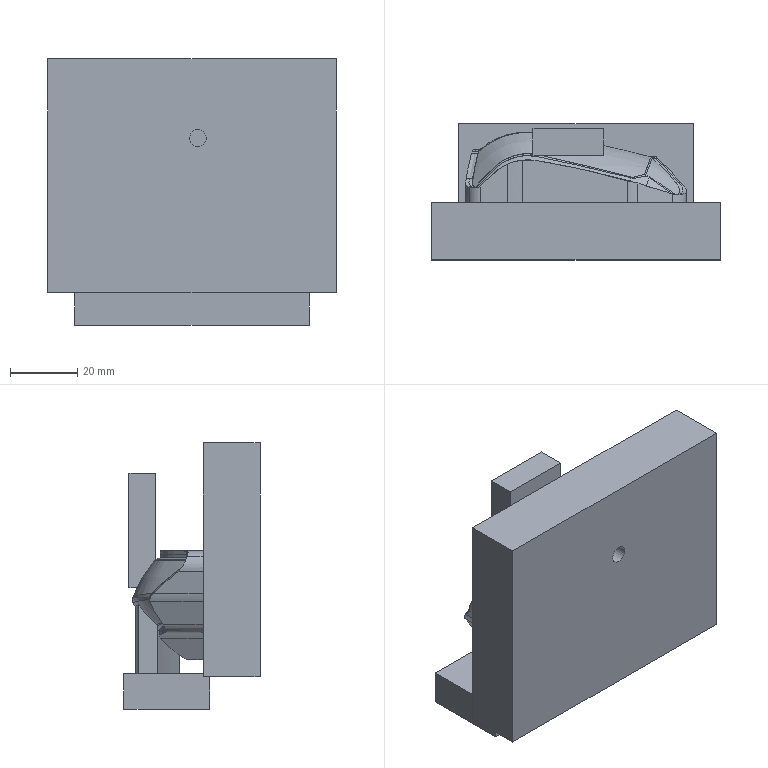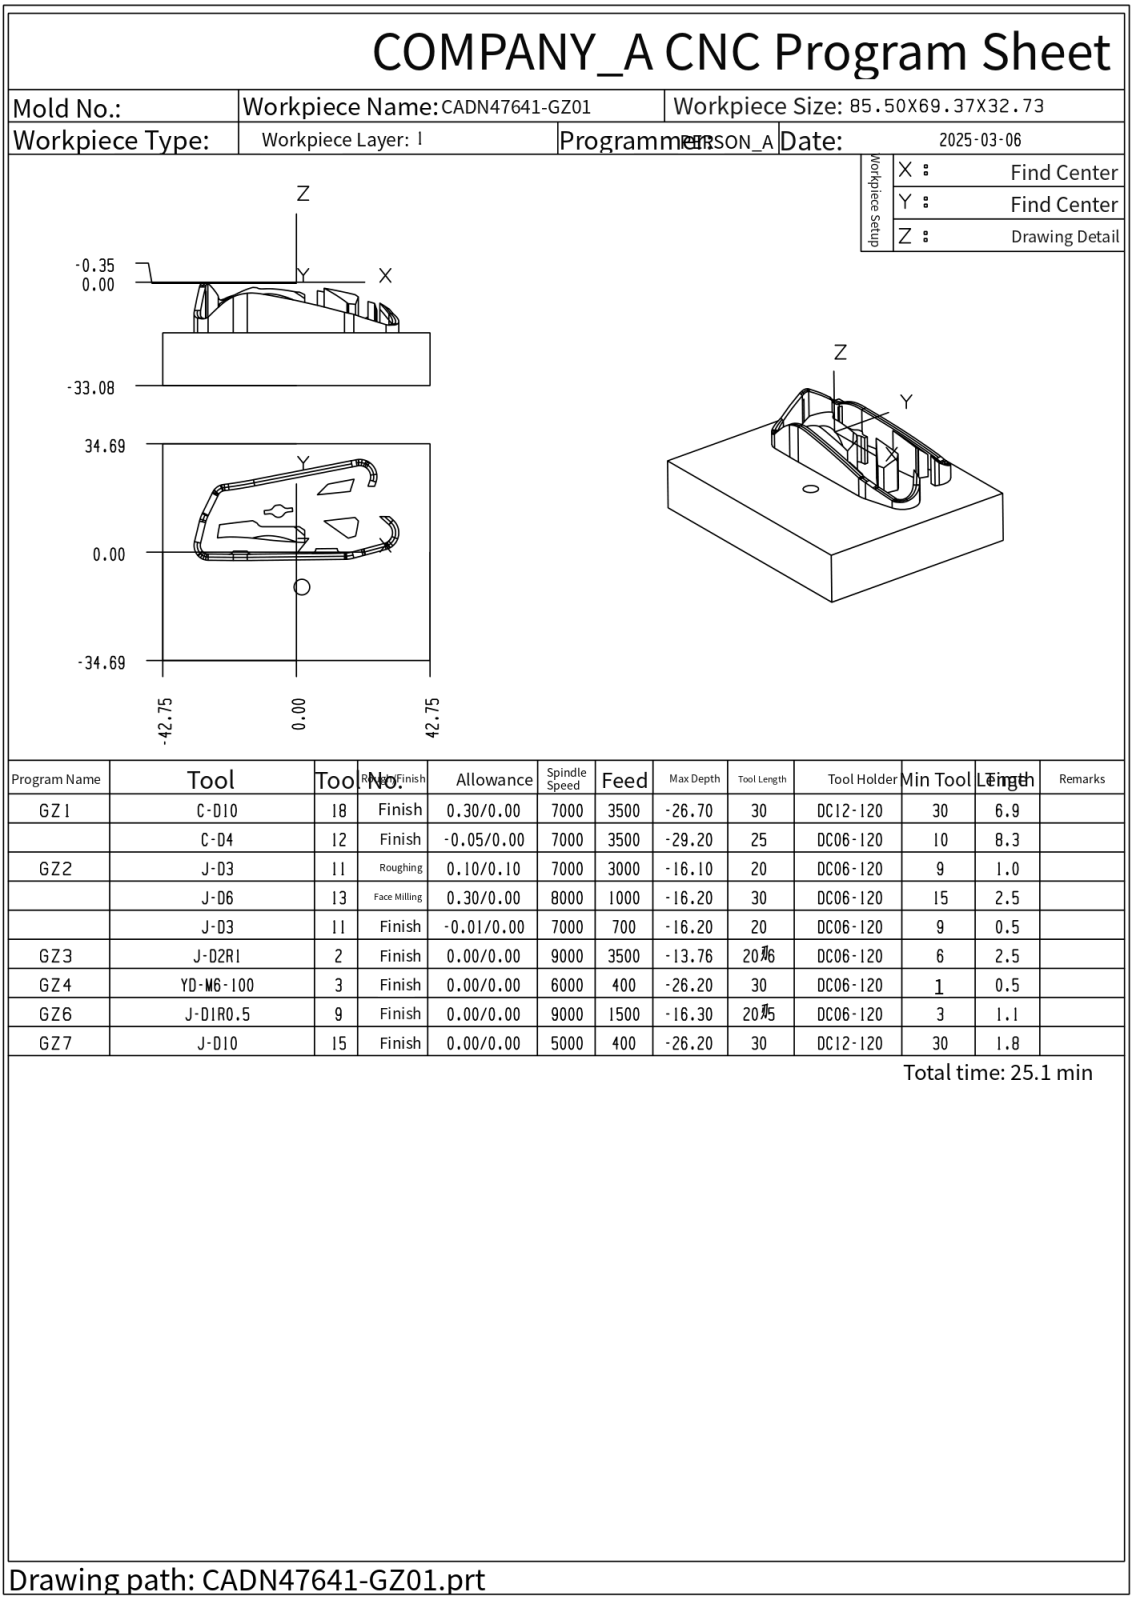NC program | NX | posted by the shop | part box 85.5 x 40.385 x 79 mm
Lines 1 to 894 of 71032:
1 BEGIN PGM A MM
2 BLK FORM 0.1 Z X-200 Y-200 Z-20
3 BLK FORM 0.2  X+200  Y+200  Z+0
4 CYCL DEF 247 DATUM SETTING ~
Q339=+1
5 * - OPERATION: 动态开粗_COPY_1 - TOOL: T14 C-D8
6 M5
7 M9
8 PLANE RESET STAY
9 CALL LBL100
10 ;(C-D8 D=8. R=0.)
11 M01
12 TOOL CALL 14 Z S7000
13 CALL LBL101
14 M3 M8
15 M51
16 CYCL DEF 7.0
17 CYCL DEF 7.1 X0
18 CYCL DEF 7.2 Y0
19 CYCL DEF 7.3 Z0
20 CYCL DEF 32.0 TOLERANCE
21 CYCL DEF 32.1 T0.096
22 CYCL DEF 32.2 HSC-MODE:0
23 L M126
24 L A+0.0 C+0.0 FMAX
25 L X-40.7663 Y-4.7564 FMAX
26 L Z5.3 FMAX
27 L Z-14.7 FMAX
28 L Z-17.7 F4000.
29 L X-40.0254 Y-4.7388
30 L X-39.2862 Y-4.6863
31 CC X-39.5061 Y-3.8936
32 C X-38.7492 Y-4.216 DR+
33 CC X-55.9353 Y-.1596
34 C X-38.2866 Y.4217 DR+
35 L X-38.2031 Y11.2888
36 CC X-33.0151 Y10.2125
37 C X-34.5468 Y15.2848 DR-
38 CC X-28.8054 Y-3.3134
39 C X-28.3228 Y16.1449 DR-
40 L X-19.7606 Y16.191
41 L X33.2624 Y16.1529
42 CC X32.3188 Y11.0031
43 C X37.3148 Y12.5687 DR-
44 CC X19.5711 Y6.8917
45 C X38.1961 Y6.4747 DR-
46 CC X-682.1256 Y-2.6235
47 C X38.2015 Y-11.2855 DR-
48 CC X33.0063 Y-10.2087
49 C X34.5482 Y-15.2853 DR-
50 CC X28.812 Y3.2985
51 C X28.3241 Y-16.1444 DR-
52 L X19.7619 Y-16.1904
53 L X-33.261 Y-16.1559
54 CC X-32.3254 Y-11.0212
55 C X-37.2907 Y-12.6294 DR-
56 CC X-19.0827 Y-6.7608
57 C X-38.1116 Y-4.7925 DR-
58 CC X-207.714 Y6.8756
59 C X-37.7288 Y9.353 DR+
60 CC X-31.4594 Y8.5945
61 C X-33.4511 Y14.5873 DR-
62 CC X-26.9702 Y-4.9504
63 C X-26.565 Y15.6302 DR-
64 L X-17.6279 Y15.6907
65 L X31.6049 Y15.6508
66 CC X30.5961 Y9.326
67 C X36.7188 Y11.2056 DR-
68 CC X15.2296 Y4.6174
69 C X37.699 Y4.0555 DR-
70 CC X-599.7023 Y-3.1683
71 C X37.708 Y-9.5448 DR-
72 CC X31.4132 Y-8.555
73 C X33.3692 Y-14.6195 DR-
74 CC X27.0224 Y4.8766
75 C X26.7268 Y-15.6245 DR-
76 L X17.9148 Y-15.69
77 L X-31.6032 Y-15.6509
78 CC X-30.5967 Y-9.3279
79 C X-36.7142 Y-11.2172 DR-
80 CC X-19.4868 Y-5.7072
81 C X-37.4871 Y-3.9371 DR-
82 CC X-490.3806 Y12.528
83 C X-37.2095 Y8.1065 DR+
84 CC X-30.1497 Y7.2716
85 C X-32.3545 Y14.0301 DR-
86 CC X-25.5192 Y-6.9093
87 C X-25.2814 Y15.1162 DR-
88 L X-15.5946 Y15.1904
89 L X30.0422 Y15.1602
90 CC X29.3483 Y8.1097
91 C X36.0839 Y10.3054 DR-
92 CC X14.3082 Y3.2829
93 C X37.1843 Y2.8563 DR-
94 CC X-145.6723 Y-2.6925
95 C X37.1816 Y-8.3282 DR-
96 CC X30.0937 Y-7.2324
97 C X32.2692 Y-14.0666 DR-
98 CC X25.3235 Y8.0785
99 C X24.9413 Y-15.1271 DR-
100 L X16.6293 Y-15.1895
101 L X-30.0076 Y-15.1621
102 CC X-29.3404 Y-8.0931
103 C X-36.1184 Y-10.2088 DR-
104 CC X-18.7292 Y-4.7615
105 C X-36.9151 Y-3.6084 DR-
106 CC X415.9145 Y-8.1786
107 C X-36.6776 Y7.1805 DR-
108 CC X-29.0112 Y6.1261
109 C X-31.3228 Y13.5113 DR-
110 CC X-23.9515 Y-10.2714
111 C X-23.5591 Y14.6244 DR-
112 L X-14.8096 Y14.6901
113 L X28.7307 Y14.6596
114 CC X28.2097 Y6.9686
115 C X35.5727 Y9.251 DR-
116 CC X11.5874 Y1.8566
117 C X36.6829 Y1.4265 DR-
118 CC X-50.2048 Y-2.5773
119 C X36.6424 Y-7.381 DR-
120 CC X29.4217 Y-6.3595
121 C X33.7793 Y-12.207 DR-
122 CC X28.8006 Y-7.969
123 C X28.4986 Y-14.5002 DR-
124 CC X16.2851 Y369.4264
125 C X14.3349 Y-14.6894 DR-
126 L X-28.7293 Y-14.6591
127 CC X-28.2374 Y-7.0359
128 C X-35.6146 Y-9.019 DR-
129 CC X-13.7801 Y-3.2089
130 C X-36.3465 Y-2.0871 DR-
131 CC X74.7165 Y-.5221
132 C X-36.143 Y6.3784 DR-
133 CC X-28.0073 Y5.1089
134 C X-30.4259 Y12.9798 DR-
135 CC X-22.9176 Y-11.3849
136 C X-22.7231 Y14.1097 DR-
137 L X-18.7621 Y14.1819
138 CC X-14.6695 Y-17.1849
139 C X-11.3073 Y14.2686 DR-
140 L X-3.2682 Y14.19
141 L X27.5437 Y14.1587
142 CC X27.1913 Y5.9618
143 C X35.034 Y8.3713 DR-
144 CC X10.7399 Y.8663
145 C X36.1661 Y.6726 DR-
146 CC X-14.8941 Y-2.4558
147 C X36.0961 Y-6.5697 DR-
148 CC X24.9679 Y-4.2662
149 C X34.9346 Y-9.7259 DR-
150 CC X30.0162 Y-8.9451
151 C X33.7793 Y-12.207 DR-
152 CC X27.4633 Y-6.4075
153 C X32.2243 Y-13.539 DR-
154 CC X28.7948 Y-7.7933
155 C X27.1899 Y-14.2893 DR-
156 CC X20.2483 Y-188.1914
157 C X16.6569 Y-14.1879 DR+
158 L X-27.605 Y-14.1543
159 CC X-27.2356 Y-6.1018
160 C X-35.0588 Y-8.0451 DR-
161 CC X-9.924 Y-1.7856
162 C X-35.8051 Y-.7347 DR-
163 CC X10.4121 Y.9456
164 C X-35.5784 Y5.8169 DR-
165 CC X-27.0618 Y4.154
166 C X-29.5438 Y12.4689 DR-
167 CC X-21.613 Y-14.237
168 C X-21.4047 Y13.6208 DR-
169 L X-18.753 Y14.1836
170 CC X-18.9034 Y14.9773
171 C X-18.1383 Y14.7179 DR+
172 L X-17.827 Y16.269 Z-17.2
173 CC X-16.3489 Y16.1626
174 C X-17.5794 Y16.9885 DR- F15000.
175 CC X-16.9632 Y16.4458
176 C X-16.9728 Y17.2668 DR-
177 L X25.1253 Y17.257
178 CC X24.4451 Y.307
179 C X33.0027 Y14.9539 DR-
180 CC X27.7346 Y6.5754
181 C X35.216 Y13.0547 DR-
182 L X35.8581 Y12.3099
183 L X36.4346 Y11.5133
184 CC X27.5189 Y6.6836
185 C X37.3339 Y9.2295 DR-
186 CC X-16.794 Y-6.0248
187 C X38.9368 Y1.4989 DR-
188 CC X12.0107 Y-1.3997
189 C X38.9758 Y-3.9093 DR-
190 CC X17.5427 Y-2.6947
191 C X37.927 Y-9.4276 DR-
192 L X37.5119 Y-10.4717
193 L X37.0272 Y-11.4853
194 L X34.8049 Y-15.6682
195 CC X33.2435 Y-14.6127
196 C X33.4874 Y-16.4815 DR-
197 L X30.1838 Y-16.8959
198 CC X30.2171 Y-16.0719
199 C X29.5003 Y-16.4796 DR-
200 L X28.6077 Y-15.1731 Z-17.7 F4000.
201 L X28.3829 Y-14.8356
202 CC X27.4191 Y-15.4567
203 C X27.7917 Y-14.3723 DR+
204 CC X21.8493 Y-39.4501
205 C X20.806 Y-13.699 DR+
206 L X-26.6046 Y-13.6478
207 CC X-26.3438 Y-5.1658
208 C X-31.624 Y-11.809 DR-
209 CC X-28.9013 Y-6.2955
210 C X-35.0393 Y-6.6662 DR-
211 CC X35.2661 Y-.4606
212 C X-35.1347 Y4.5478 DR-
213 CC X-26.2559 Y3.3262
214 C X-28.928 Y11.881 DR-
215 CC X-21.6436 Y-10.4001
216 C X-23.4569 Y12.9713 DR-
217 L X-21.2944 Y13.647
218 CC X-21.5142 Y14.4164
219 C X-21.0775 Y15.0869 DR+
220 L X-21.4377 Y15.2114 Z-17.5793
221 L X-21.8174 Y15.2442 Z-17.4585
222 L X-22.6307 Y15.3116 Z-17.2
223 L X-24.2701 Y15.4401 F15000.
224 L X-30.4912 Y14.2495
225 CC X-29.1866 Y9.2641
226 C X-32.8263 Y12.9122 DR+
227 L X-35.4759 Y10.2463
228 CC X-29.0644 Y4.843
229 C X-37.2266 Y6.7617 DR+
230 L X-37.3789 Y5.9892
231 L X-37.4691 Y5.2071
232 L X-38.121 Y-5.0097
233 L X-38.0578 Y-5.2475
234 L X-37.9314 Y-5.4586
235 L X-37.0448 Y-6.492
236 L X-36.6866 Y-6.92 Z-17.3769 F4000.
237 L X-36.2979 Y-7.3206 Z-17.5539
238 L X-36.0913 Y-7.4228 Z-17.6269
239 L X-35.8653 Y-7.4681 Z-17.7
240 CC X-35.8404 Y-6.6673
241 C X-35.0393 Y-6.6662 DR+
242 CC X34.85 Y-6.4364
243 C X-34.8414 Y-1.1759 DR-
244 CC X-3.739 Y-.2793
245 C X-34.4537 Y4.698 DR-
246 CC X-25.4356 Y2.4811
247 C X-28.2498 Y11.3309 DR-
248 CC X-12.4433 Y-40.2752
249 C X-25.6036 Y12.0683 DR-
250 L X-23.4212 Y12.9855
251 CC X-23.7182 Y13.7289
252 C X-23.0891 Y14.224 DR+
253 CC X-23.8201 Y13.5658
254 CP IPA49.2089 IZ.267 DR+
255 L X-24.5706 Y14.6369 Z-17.2
256 L X-26.2393 Y14.8255 F15000.
257 L X-26.5045 Y14.7656
258 L X-28.3336 Y14.016
259 L X-30.143 Y13.2197
260 CC X-22.0304 Y-2.4672
261 C X-32.6486 Y11.6448 DR+
262 L X-35.7878 Y9.275
263 CC X-33.6594 Y6.9518
264 C X-36.7623 Y7.4988 DR+
265 L X-36.9093 Y6.7247
266 L X-37.001 Y5.942
267 L X-37.4739 Y-.944
268 L X-37.4194 Y-1.1766
269 L X-36.8534 Y-2.5948
270 L X-36.6431 Y-3.1359 Z-17.3839 F4000.
271 L X-36.4025 Y-3.6642 Z-17.5678
272 L X-36.2601 Y-3.8166 Z-17.6339
273 L X-36.0877 Y-3.9341 Z-17.7
274 CC X-35.7467 Y-3.2098
275 C X-34.957 Y-3.3417 DR+
276 CC X-95.281 Y7.4575
277 C X-34.1664 Y2.9174 DR+
278 CC X-24.8368 Y1.7566
279 C X-28.5505 Y10.3936 DR-
280 CC X-5.1557 Y-27.3457
281 C X-25.5641 Y12.0887 DR-
282 CC X-25.931 Y12.7997
283 C X-25.7957 Y13.5883 DR+
284 L X-26.239 Y13.5657 Z-17.5596
285 L X-26.6749 Y13.4819 Z-17.4191
286 L X-27.3571 Y13.3626 Z-17.2
287 L X-28.8095 Y13.1016 F15000.
288 L X-29.003 Y13.0102
289 L X-30.6631 Y11.9398
290 L X-32.3017 Y10.837
291 CC X-27.4738 Y3.7511
292 C X-34.4105 Y8.791 DR+
293 L X-36.2365 Y6.1486
294 CC X-31.4664 Y3.2682
295 C X-37.0354 Y3.4604 DR+
296 L X-37.1068 Y1.0941
297 L X-37.0542 Y.8809
298 L X-36.4739 Y-.5734
299 L X-36.2686 Y-1.1046 Z-17.3804 F4000.
300 L X-36.0291 Y-1.6211 Z-17.5609
301 L X-35.8769 Y-1.7793 Z-17.6304
302 L X-35.6912 Y-1.8963 Z-17.7
303 CC X-35.379 Y-1.159
304 C X-34.5933 Y-1.3134 DR+
305 CC X191.8774 Y-48.2763
306 C X-33.0672 Y5.5237 DR-
307 CC X-26.8533 Y3.5659
308 C X-30.6668 Y8.8482 DR-
309 L X-28.5134 Y10.4171
310 CC X-28.9516 Y11.1003
311 C X-28.1409 Y11.0606 DR+
312 L X-28.1264 Y11.4112
313 L X-28.0609 Y12.9921 Z-17.2
314 CC X-27.199 Y13.0835
315 C X-27.5919 Y13.856 DR- F15000.
316 L X-25.8007 Y14.6886
317 L X-23.9766 Y15.4466
318 L X-22.0978 Y16.0478
319 L X-18.6454 Y16.9835
320 CC X-17.348 Y10.7796
321 C X-16.4517 Y17.054 DR-
322 L X-15.0389 Y16.8387
323 CC X-15.3571 Y15.9443
324 C X-14.5454 Y16.4366 DR-
325 L X-13.587 Y15.1775 Z-17.7 F4000.
326 L X-13.3178 Y14.8112
327 CC X-12.2693 Y15.5782
328 C X-12.1023 Y14.2899 DR+
329 CC X-4.5087 Y61.1648
330 C X-3.1268 Y13.6989 DR+
331 L X26.5567 Y13.6515
332 CC X26.2407 Y5.0131
333 C X34.5271 Y7.4744 DR-
334 CC X7.523 Y-.5046
335 C X35.6782 Y-.9132 DR-
336 CC X14.7805 Y-2.6586
337 C X35.3706 Y-6.6345 DR-
338 CC X39.8744 Y-8.4523
339 C X35.0367 Y-8.8825 DR+
340 L X34.9315 Y-9.7511
341 CC X35.7264 Y-9.8466
342 C X35.8525 Y-10.6372 DR+
343 CC X35.6328 Y-9.6765
344 CP IPA49.0063 IZ.2664 DR+
345 L X36.9368 Y-9.5459 Z-17.2
346 L X37.9398 Y-8.1622 F15000.
347 CC X28.4918 Y-4.9219
348 C X38.4657 Y-5.4567 DR+
349 L X38.3881 Y-2.2962
350 L X38.2386 Y.8618
351 CC X-14.1945 Y-3.6796
352 C X37.2346 Y7.4962 DR+
353 CC X25.3859 Y4.0871
354 C X35.6338 Y10.9424 DR+
355 CC X26.7332 Y5.5742
356 C X33.818 Y13.1797 DR+
357 CC X23.5877 Y1.666
358 C X31.6721 Y14.7758 DR+
359 CC X27.4702 Y7.1763
360 C X28.6118 Y15.7848 DR+
361 CC X25.0197 Y-6.3379
362 C X25.3403 Y16.0722 DR+
363 L X-7.1504 Y16.4323
364 L X-7.3469 Y16.3837
365 L X-8.7935 Y15.824
366 L X-9.3469 Y15.6141 Z-17.3875 F4000.
367 L X-9.8898 Y15.3783 Z-17.575
368 L X-10.0374 Y15.2473 Z-17.6375
369 L X-10.1562 Y15.0897 Z-17.7
370 CC X-9.4505 Y14.7121
371 C X-9.5666 Y13.9201 DR+
372 CC X-1.7128 Y55.5265
373 C X-.4953 Y13.2028 DR+
374 L X25.494 Y13.153
375 CC X25.3617 Y4.1573
376 C X33.9666 Y6.7834 DR-
377 CC X7.2013 Y-1.3173
378 C X35.1642 Y-1.5974 DR-
379 CC X11.69 Y-2.337
380 C X34.8957 Y-5.9538 DR-
381 CC X27.4719 Y-7.4359
382 C X35.0307 Y-7.8536 DR-
383 CC X35.8308 Y-7.8487
384 C X36.4175 Y-8.3927 DR+
385 L X36.6134 Y-8.0448 Z-17.5736
386 L X36.7395 Y-7.666 Z-17.4472
387 L X36.9935 Y-6.9275 Z-17.2
388 L X37.5481 Y-5.3362 F15000.
389 L X37.8823 Y-4.6836
390 L X38.1696 Y-4.0091
391 CC X35.2214 Y-3.0935
392 C X38.2675 Y-2.592 DR+
393 L X37.0983 Y4.2382
394 CC X11.0586 Y-1.0107
395 C X35.7658 Y8.7449 DR+
396 L X34.9853 Y10.6848
397 CC X30.0915 Y8.2343
398 C X33.4715 Y12.5389 DR+
399 L X32.5225 Y13.2428
400 L X31.4235 Y13.9649
401 L X30.2957 Y14.6414
402 CC X27.1767 Y7.9273
403 C X28.1016 Y15.2725 DR+
404 CC X21.7578 Y-36.4835
405 C X22.1874 Y15.658 DR+
406 L X-4.329 Y15.974
407 L X-4.5277 Y15.9244
408 L X-5.964 Y15.3627
409 L X-6.5145 Y15.1521 Z-17.3867 F4000.
410 L X-7.0538 Y14.9144 Z-17.5734
411 L X-7.2023 Y14.7807 Z-17.6367
412 L X-7.3207 Y14.6197 Z-17.7
413 CC X-6.6102 Y14.2511
414 C X-6.7441 Y13.4618 DR+
415 CC X1.4996 Y56.436
416 C X2.8744 Y12.6999 DR+
417 L X24.4928 Y12.6537
418 CC X24.4724 Y3.2499
419 C X33.5333 Y5.7663 DR-
420 CC X6.2909 Y-2.047
421 C X34.5125 Y-4.6428 DR-
422 CC X14.7583 Y-11.0888
423 C X34.9019 Y-5.9886 DR-
424 CC X35.6899 Y-5.8461
425 C X35.983 Y-6.5912 DR+
426 CC X35.5585 Y-5.7021
427 CP IPA51.4959 IZ.2799 DR+
428 L X36.7714 Y-5.2774 Z-17.2
429 L X37.3948 Y-3.6681 F15000.
430 L X37.4194 Y-3.4711
431 L X37.4187 Y-1.4969
432 L X37.3222 Y.4751
433 CC X12.8536 Y-2.1851
434 C X35.2372 Y8.0503 DR+
435 CC X14.1512 Y-2.2984
436 C X33.4031 Y11.1582 DR+
437 CC X26.8495 Y5.7527
438 C X30.8856 Y13.2279 DR+
439 CC X23.6068 Y1.5087
440 C X28.4479 Y14.4271 DR+
441 CC X24.8018 Y2.9539
442 C X25.3527 Y14.9799 DR+
443 L X23.8728 Y15.0665
444 L X22.3915 Y15.121
445 L X-1.4335 Y15.4854
446 L X-1.6342 Y15.4355
447 L X-3.0811 Y14.869
448 L X-3.627 Y14.6605 Z-17.3851 F4000.
449 L X-4.161 Y14.423 Z-17.5703
450 L X-4.3122 Y14.285 Z-17.6351
451 L X-4.4307 Y14.118 Z-17.7
452 CC X-3.7136 Y13.7623
453 C X-3.8475 Y12.973 DR+
454 CC X4.1378 Y52.8318
455 C X5.4413 Y12.2019 DR+
456 CC X11.5026 Y-847.4596
457 C X23.9189 Y12.1336 DR-
458 CC X23.7031 Y2.4896
459 C X32.9862 Y5.112 DR-
460 CC X6.4702 Y-2.5245
461 C X34.0437 Y-3.5809 DR-
462 L X34.5369 Y-4.7444
463 CC X35.2925 Y-4.4755
464 C X35.4589 Y-5.26 DR+
465 CC X35.1964 Y-4.3433
466 CP IPA58.1597 IZ.3063 DR+
467 L X36.3686 Y-4.0493 Z-17.2
468 L X37.0337 Y-2.581 F15000.
469 L X37.0544 Y-2.227
470 L X36.2627 Y2.4519
471 CC X14.5894 Y-1.5622
472 C X34.6381 Y7.5973 DR+
473 CC X14.3605 Y-2.3028
474 C X32.9621 Y10.471 DR+
475 CC X26.8398 Y5.5569
476 C X30.8733 Y12.2921 DR+
477 CC X20.8896 Y-3.491
478 C X28.2686 Y13.6651 DR+
479 CC X24.1073 Y2.76
480 C X25.1285 Y14.3873 DR+
481 L X23.555 Y14.5291
482 L X21.9769 Y14.6031
483 L X1.1424 Y15.0222
484 L X.9372 Y14.971
485 L X-.5162 Y14.3951
486 L X-1.0527 Y14.1888 Z-17.3821 F4000.
487 L X-1.5756 Y13.9501 Z-17.5643
488 L X-1.7314 Y13.8031 Z-17.6321
489 L X-1.8492 Y13.6242 Z-17.7
490 CC X-1.1189 Y13.296
491 C X-1.2692 Y12.5096 DR+
492 CC X6.5354 Y49.0093
493 C X7.7574 Y11.7045 DR+
494 CC X11.9028 Y-645.7099
495 C X23.2435 Y11.6197 DR-
496 CC X22.9686 Y1.7785
497 C X32.4056 Y4.5838 DR-
498 CC X8.5408 Y-2.7494
499 C X33.5054 Y-2.4778 DR-
500 CC X35.2008 Y-2.2677
501 C X33.8722 Y-3.3417 DR+
502 L X34.1261 Y-3.8436
503 CC X34.8402 Y-3.4813
504 C X35.3169 Y-4.1247 DR+
505 CC X34.6816 Y-3.3812
506 CP IPA52.3235 IZ.2823 DR+
507 L X35.7252 Y-2.6499 Z-17.2
508 L X35.9062 Y-.7603 F15000.
509 CC X23.5859 Y-.2211
510 C X35.7524 Y1.793 DR+
511 CC X9.5588 Y-3.6898
512 C X33.3963 Y8.4733 DR+
513 CC X26.4071 Y4.5794
514 C X31.3689 Y10.8557 DR+
515 CC X21.6219 Y-.5756
516 C X28.9545 Y12.5359 DR+
517 CC X23.0308 Y1.0741
518 C X23.299 Y13.9734 DR+
519 L X3.7802 Y14.5208
520 L X3.5703 Y14.4689
521 L X2.1206 Y13.8929
522 L X1.5851 Y13.6864 Z-17.3819 F4000.
523 L X1.0634 Y13.4472 Z-17.5637
524 L X.9073 Y13.2993 Z-17.6319
525 L X.7897 Y13.1193 Z-17.7
526 CC X1.5213 Y12.794
527 C X1.371 Y12.0076 DR+
528 CC X9.1378 Y48.3127
529 C X10.3205 Y11.205 DR+
530 CC X13.8953 Y-274.2944
531 C X22.8048 Y11.0883 DR-
532 CC X22.2447 Y1.0483
533 C X31.8998 Y3.8584 DR-
534 CC X1.0413 Y-4.9105
535 C X32.9813 Y-1.915 DR-
536 CC X39.2219 Y1.1546
537 C X33.6443 Y-2.9996 DR+
538 CC X34.3107 Y-2.5539
539 C X34.6988 Y-3.2554 DR+
540 CC X34.1815 Y-2.4564
541 CP IPA58.3914 IZ.307 DR+
542 L X35.2127 Y-1.8315 Z-17.2
543 L X35.4383 Y-.0434 F15000.
544 L X35.0938 Y1.8668
545 L X34.6881 Y3.7649
546 CC X23.2004 Y.3273
547 C X33.3979 Y6.6358 DR+
548 L X32.609 Y7.9523
549 L X31.7701 Y9.2376
550 CC X24.7486 Y3.9465
551 C X29.5736 Y11.2961 DR+
552 CC X22.0616 Y.8022
553 C X27.3553 Y12.572 DR+
554 CC X23.6617 Y3.4411
555 C X25.0785 Y13.1884 DR+
556 CC X18.8896 Y-25.3917
557 C X20.1641 Y13.6609 DR+
558 L X6.3594 Y14.0305
559 L X6.1501 Y13.9786
560 L X4.7131 Y13.4079
561 L X4.1729 Y13.1992 Z-17.3835 F4000.
562 L X3.6458 Y12.9596 Z-17.5669
563 L X3.4923 Y12.8162 Z-17.6335
564 L X3.3746 Y12.6423 Z-17.7
565 CC X4.1001 Y12.3037
566 C X3.9498 Y11.5174 DR+
567 CC X11.213 Y43.2282
568 C X12.2065 Y10.7114 DR+
569 CC X14.5479 Y-179.8692
570 C X22.1679 Y10.5734 DR-
571 CC X21.5494 Y.3706
572 C X31.3815 Y3.1651 DR-
573 CC X-53.5664 Y-19.0741
574 C X32.4384 Y-1.3571 DR-
575 L X33.1006 Y-2.2135
576 CC X33.7233 Y-1.7074
577 C X34.0944 Y-2.4188 DR+
578 CC X33.5952 Y-1.6064
579 CP IPA58.1637 IZ.3063 DR+
580 L X34.6452 Y-1.0081 Z-17.2
581 L X34.9043 Y.6564 F15000.
582 L X34.795 Y1.2479
583 L X34.6408 Y1.8292
584 L X34.3587 Y2.7742
585 L X34.0056 Y3.6951
586 L X32.6372 Y6.8069
587 CC X24.1653 Y2.537
588 C X29.6842 Y10.2537 DR+
589 CC X21.3723 Y-1.0236
590 C X22.7439 Y12.9186 DR+
591 L X21.1717 Y13.0796
592 L X19.5943 Y13.1766
593 L X8.6391 Y13.564
594 L X8.4232 Y13.5105
595 L X6.9931 Y12.9353
596 L X6.4583 Y12.7266 Z-17.3819 F4000.
597 L X5.9374 Y12.4852 Z-17.5639
598 L X5.782 Y12.3368 Z-17.6319
599 L X5.6652 Y12.1565 Z-17.7
600 CC X6.398 Y11.8338
601 C X6.233 Y11.0503 DR+
602 CC X13.5217 Y41.8512
603 C X14.4592 Y10.2135 DR+
604 CC X16.2513 Y-57.4061
605 C X22.2954 Y9.9667 DR-
606 CC X20.919 Y-.2465
607 C X30.8218 Y2.6064 DR-
608 CC X77.4702 Y14.9509
609 C X31.7925 Y-.6057 DR+
610 L X32.535 Y-1.5141
611 CC X33.1579 Y-1.0077
612 C X33.5038 Y-1.7321 DR+
613 CC X33.0347 Y-.9041
614 CP IPA58.4191 IZ.3071 DR+
615 L X34.1005 Y-.3409 Z-17.2
616 L X34.388 Y1.2069 F15000.
617 L X34.3646 Y1.3907
618 L X34.3152 Y1.5691
619 L X33.4883 Y3.3631
620 L X32.5893 Y5.122
621 CC X17.7794 Y-2.9039
622 C X29.7502 Y8.9472 DR+
623 CC X21.7678 Y.9672
624 C X24.4483 Y11.9314 DR+
625 CC X19.0354 Y-9.5705
626 C X20.3719 Y12.562 DR+
627 L X15.6981 Y12.8487
628 L X11.0206 Y13.0656
629 L X10.7965 Y13.0109
630 L X9.3787 Y12.4376
631 L X8.8436 Y12.2276 Z-17.3821 F4000.
632 L X8.3224 Y11.9851 Z-17.5643
633 L X8.1677 Y11.8371 Z-17.6321
634 L X8.0512 Y11.6574 Z-17.7
635 CC X8.7837 Y11.3342
636 C X8.6188 Y10.5507 DR+
637 CC X15.5434 Y38.7487
638 C X16.2268 Y9.721 DR+
639 CC X17.2907 Y-19.7095
640 C X22.99 Y9.1835 DR-
641 CC X20.204 Y-.9567
642 C X30.2272 Y2.2245 DR-
643 L X30.9159 Y.4384
644 L X31.8316 Y-.6532
645 CC X32.449 Y-.1434
646 C X33.091 Y-.6217 DR+
647 CC X32.2513 Y-.086
648 CP IPA50.3121 IZ.2765 DR+
649 L X33.0846 Y.9132 Z-17.2
650 L X32.9389 Y1.853 F15000.
651 L X32.7531 Y2.7857
652 L X32.2358 Y4.0482
653 L X31.6683 Y5.2889
654 CC X23.4579 Y.8779
655 C X30.0623 Y7.4543 DR+
656 L X29.0092 Y8.5176
657 L X27.9169 Y9.5406
658 CC X22.1984 Y2.5699
659 C X25.3005 Y11.0356 DR+
660 CC X19.9173 Y-2.1472
661 C X22.8519 Y11.7868 DR+
662 L X21.6767 Y11.9426
663 L X20.497 Y12.0585
664 L X13.2479 Y12.5892
665 L X13.008 Y12.5318
666 L X11.5839 Y11.9465
667 L X11.0616 Y11.739 Z-17.3781 F4000.
668 L X10.5552 Y11.4951 Z-17.5563
669 L X10.3951 Y11.3345 Z-17.6281
670 L X10.2807 Y11.1388 Z-17.7
671 CC X11.0291 Y10.8536
672 C X10.8541 Y10.0722 DR+
673 CC X17.7291 Y36.7658
674 C X18.1133 Y9.2037 DR+
675 CC X18.3911 Y-5.1913
676 C X24.8691 Y7.6667 DR-
677 CC X18.6458 Y-2.4009
678 C X29.7088 Y1.8059 DR-
679 L X30.926 Y.4271
680 CC X31.5216 Y.9626
681 C X32.1049 Y.4137 DR+
682 CC X31.3706 Y1.0205
683 CP IPA55.4503 IZ.2916 DR+
684 L X32.2024 Y1.933 Z-17.2
685 L X31.9716 Y3.6227 F15000.
686 L X31.8474 Y3.866
687 L X29.2062 Y7.3698
688 CC X22.4915 Y1.7808
689 C X26.5328 Y9.5262 DR+
690 CC X18.8989 Y-3.893
691 C X21.2777 Y11.3613 DR+
692 L X18.2687 Y11.7748
693 L X15.2517 Y12.1257
694 L X14.9817 Y12.0637
695 L X13.6104 Y11.4849
696 L X13.0868 Y11.2708 Z-17.3793 F4000.
697 L X12.579 Y11.0217 Z-17.5585
698 L X12.4221 Y10.8629 Z-17.6293
699 L X12.3092 Y10.6704 Z-17.7
700 CC X13.0566 Y10.3828
701 C X12.8732 Y9.6033 DR+
702 CC X20.9863 Y41.2613
703 C X19.4006 Y8.6187 DR+
704 CC X18.7125 Y-2.4052
705 C X28.1077 Y3.4026 DR-
706 L X29.7841 Y1.6937
707 CC X30.3721 Y2.2362
708 C X31.1605 Y2.3723 DR+
709 L X30.9498 Y2.8961 Z-17.5214
710 L X30.6932 Y3.399 Z-17.3428
711 L X30.4944 Y3.8045 Z-17.2
712 L X29.1865 Y6.4238 F15000.
713 CC X24.8392 Y3.7891
714 C X27.7491 Y7.9572 DR+
715 CC X17.1527 Y-6.9866
716 C X23.5988 Y10.1612 DR+
717 L X22.7956 Y10.4123
718 L X21.982 Y10.6274
719 L X17.3946 Y11.6401
720 L X17.2059 Y11.6209
721 L X17.0223 Y11.5729
722 L X15.7126 Y10.9925
723 L X15.1957 Y10.7707 Z-17.3783 F4000.
724 L X14.6957 Y10.5131 Z-17.5566
725 L X14.5402 Y10.3486 Z-17.6283
726 L X14.4311 Y10.1504 Z-17.7
727 CC X15.1866 Y9.8845
728 C X15.0031 Y9.1049 DR+
729 L X21.1974 Y7.7195
730 CC X13.9091 Y-15.3444
731 C X24.4672 Y6.4177 DR-
732 CC X7.5573 Y-17.7001
733 C X28.1463 Y3.3643 DR-
734 CC X28.7102 Y3.932
735 C X29.4977 Y3.7902 DR+
736 CC X28.2791 Y3.8902
737 CP IPA35.8365 IZ.2418 DR+
738 L X29.0003 Y5.2703 Z-17.2
739 L X28.3775 Y6.6821 F15000.
740 L X28.1463 Y6.9245
741 L X26.6329 Y7.9575
742 L X25.0715 Y8.9164
743 L X24.0639 Y9.4161
744 L X23.028 Y9.8541
745 L X19.7074 Y11.1043
746 L X19.4475 Y11.1104
747 L X19.1976 Y11.0389
748 L X17.9797 Y10.4437
749 L X17.4782 Y10.2063 Z-17.3759 F4000.
750 L X16.9961 Y9.9317 Z-17.5518
751 L X16.8439 Y9.7543 Z-17.6259
752 L X16.7439 Y9.543 Z-17.7
753 CC X17.5153 Y9.3264
754 C X17.3155 Y8.5505 DR+
755 CC X46.3771 Y110.0683
756 C X23.2527 Y7.0358 DR+
757 L X24.1058 Y7.3744
758 L X25.5409 Y8.0408 Z-17.2
759 CC X25.9294 Y7.3265
760 C X26.4125 Y7.9806 DR- F15000.
761 L X30.0952 Y5.2036
762 CC X17.0216 Y-10.6204
763 C X33.9051 Y1.0528 DR-
764 L X35.2587 Y-1.0129
765 L X36.553 Y-3.1163
766 CC X28.847 Y-7.4064
767 C X37.6436 Y-8.0443 DR-
768 L X36.9833 Y-12.4536
769 CC X33.892 Y-11.6939
770 C X35.8966 Y-14.1666 DR-
771 L X35.2819 Y-14.6559
772 L X34.6212 Y-15.0813
773 L X31.0422 Y-17.0876
774 CC X29.7876 Y-14.3486
775 C X29.3951 Y-17.3355 DR-
776 L X28.2768 Y-17.1745
777 CC X28.5196 Y-16.4007
778 C X27.7452 Y-16.6415 DR-
779 L X27.6704 Y-16.3948
780 L X27.2114 Y-14.8805 Z-17.7 F4000.
781 CC X26.2129 Y-15.028
782 C X26.7421 Y-14.1685 DR+
783 CC X21.5421 Y-28.4068
784 C X21.1527 Y-13.2536 DR+
785 L X14.894 Y-13.1895
786 L X-25.3057 Y-13.1615
787 CC X-24.8472 Y-.8523
788 C X-29.1473 Y-12.3951 DR-
789 CC X-29.3418 Y-7.6619
790 C X-31.6746 Y-11.7849 DR-
791 CC X-32.0531 Y-12.5793
792 C X-32.0834 Y-13.4588 DR+
793 L X-27.2884 Y-13.6239
794 L X-25.707 Y-13.6783 Z-17.2
795 L X24.1199 Y-15.3936 F15000.
796 L X24.6898 Y-15.4177 Z-17.3807 F4000.
797 L X25.2601 Y-15.4105 Z-17.5614
798 L X25.4678 Y-15.3417 Z-17.6307
799 L X25.6565 Y-15.231 Z-17.7
800 CC X25.1025 Y-14.547
801 C X25.3768 Y-13.7106 DR+
802 CC X19.7897 Y-29.572
803 C X19.4031 Y-12.7598 DR+
804 L X10.7693 Y-12.6897
805 L X-24.4927 Y-12.6532
806 CC X-16.6232 Y60.859
807 C X-27.6166 Y-12.2513 DR-
808 CC X-29.5669 Y.3667
809 C X-29.1622 Y-12.3948 DR-
810 CC X-29.1827 Y-13.2745
811 C X-29.1965 Y-14.1544 DR+
812 L X-28.8964 Y-14.1591
813 L X-27.3143 Y-14.1838 Z-17.2
814 L X22.8228 Y-14.9655 F15000.
815 L X23.3744 Y-14.9797 Z-17.3748 F4000.
816 L X23.9256 Y-14.9564 Z-17.5497
817 L X24.1474 Y-14.8725 Z-17.6248
818 L X24.3426 Y-14.7379 Z-17.7
819 CC X23.7363 Y-14.0997
820 C X24.0107 Y-13.2633 DR+
821 CC X18.0874 Y-30.2918
822 C X17.7747 Y-12.2652 DR+
823 L X10.519 Y-12.19
824 L X-23.6804 Y-12.1469
825 CC X-27.7714 Y-46.2404
826 C X-26.5709 Y-11.9233 DR+
827 L X-27.6166 Y-12.2513
828 CC X-27.4039 Y-13.1055
829 C X-28.0685 Y-13.6828 DR+
830 CC X-27.3216 Y-12.9507
831 CP IPA53.1036 IZ.3066 DR+
832 L X-26.5746 Y-13.9937 Z-17.2
833 L X21.1316 Y-14.4697 F15000.
834 L X21.739 Y-14.4839 Z-17.3925 F4000.
835 L X22.3457 Y-14.4517 Z-17.585
836 L X22.5149 Y-14.3859 Z-17.6425
837 L X22.6736 Y-14.2979 Z-17.7
838 CC X22.1376 Y-13.5998
839 C X22.393 Y-12.7575 DR+
840 CC X15.7761 Y-33.6321
841 C X15.1872 Y-11.7417 DR+
842 L X9.3936 Y-11.6905
843 L X-22.7426 Y-11.65
844 CC X-24.9004 Y-30.1061
845 C X-25.8226 Y-11.5472 DR+
846 L X-26.6273 Y-11.9417
847 CC X-26.3528 Y-12.7784
848 C X-27.0966 Y-13.2497 DR+
849 CC X-26.2728 Y-12.6535
850 CP IPA62.4753 IZ.3511 DR+
851 L X-25.656 Y-13.6626 Z-17.2
852 L X19.3718 Y-13.9531 F15000.
853 L X19.9424 Y-13.9612 Z-17.3808 F4000.
854 L X20.5127 Y-13.9382 Z-17.5616
855 L X20.7181 Y-13.8638 Z-17.6308
856 L X20.9035 Y-13.7482 Z-17.7
857 CC X20.3313 Y-13.0793
858 C X20.5745 Y-12.2334 DR+
859 CC X14.5535 Y-30.3773
860 C X14.2181 Y-11.2634 DR+
861 L X6.2081 Y-11.1894
862 L X-21.929 Y-11.1512
863 CC X-23.5644 Y-25.6601
864 C X-25.129 Y-11.1433 DR+
865 L X-25.8966 Y-11.5766
866 CC X-25.4809 Y-12.3537
867 C X-26.2737 Y-12.7386 DR+
868 CC X-25.4473 Y-12.3094
869 CP IPA69.3555 IZ.3562 DR+
870 L X-24.8836 Y-13.237 Z-17.2
871 L X18.0509 Y-13.5074 F15000.
872 L X18.5863 Y-13.5195 Z-17.3697 F4000.
873 L X19.1202 Y-13.4775 Z-17.5394
874 L X19.349 Y-13.3685 Z-17.6197
875 L X19.5426 Y-13.205 Z-17.7
876 CC X18.8736 Y-12.6327
877 C X19.1412 Y-11.794 DR+
878 CC X13.4461 Y-27.2071
879 C X13.0711 Y-10.7798 DR+
880 L X5.831 Y-10.6904
881 L X-20.993 Y-10.6593
882 CC X-22.4772 Y-27.8479
883 C X-24.293 Y-10.6911 DR+
884 L X-25.2899 Y-11.2267
885 CC X-24.7494 Y-11.9236
886 C X-25.5232 Y-12.3467 DR+
887 CC X-24.6834 Y-11.8273
888 CP IPA66.5016 IZ.3628 DR+
889 L X-24.1099 Y-12.8075 Z-17.2
890 L X16.7987 Y-13.085 F15000.
891 L X17.3436 Y-13.0946 Z-17.3727 F4000.
892 L X17.8877 Y-13.0647 Z-17.5455
893 L X18.1142 Y-12.9744 Z-17.6227